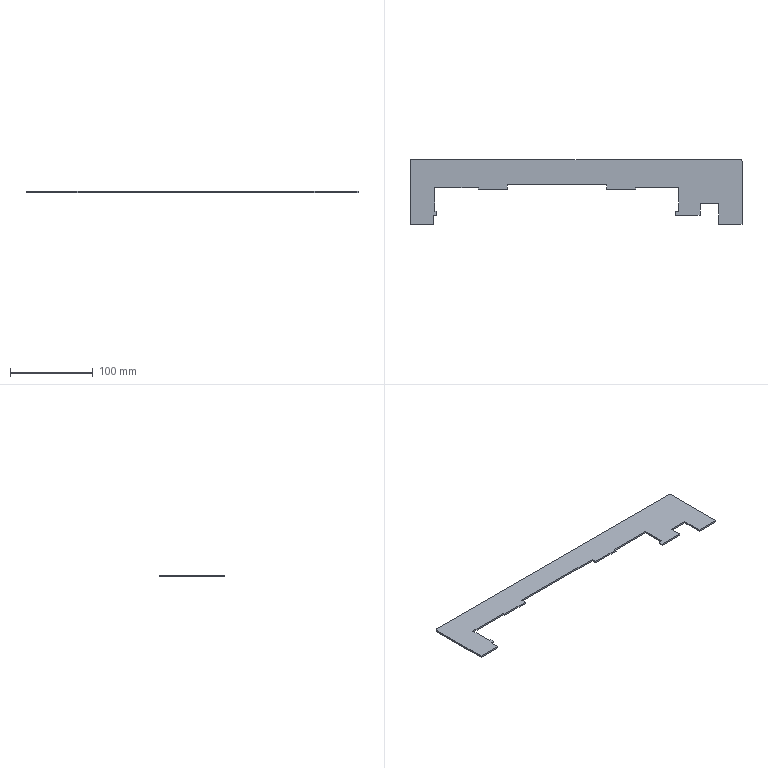Part | STEP file | xzz-001-1 | 1 solid | 30 faces | box 400 x 78 x 2 mm | volume 34179 mm3 | plane 28 | cylinder 2 | commonest cylinder face diameters 4 x2
STEP:
#1=CARTESIAN_POINT('',(221.,30.,0.));
#2=VERTEX_POINT('',#1);
#3=CARTESIAN_POINT('',(223.,28.,0.));
#4=VERTEX_POINT('',#3);
#5=CARTESIAN_POINT('',(221.,28.,0.));
#6=DIRECTION('',(0.,0.,-1.));
#7=DIRECTION('',(1.,0.,0.));
#8=AXIS2_PLACEMENT_3D('',#5,#6,#7);
#9=CIRCLE('',#8,2.);
#10=EDGE_CURVE('',#2,#4,#9,.T.);
#11=ORIENTED_EDGE('',*,*,#10,.F.);
#12=CARTESIAN_POINT('',(-175.,30.,0.));
#13=VERTEX_POINT('',#12);
#14=CARTESIAN_POINT('',(0.,30.,0.));
#15=DIRECTION('',(1.,0.,0.));
#16=VECTOR('',#15,1000.);
#17=LINE('',#14,#16);
#18=EDGE_CURVE('',#13,#2,#17,.T.);
#19=ORIENTED_EDGE('',*,*,#18,.F.);
#20=CARTESIAN_POINT('',(-177.,28.,0.));
#21=VERTEX_POINT('',#20);
#22=CARTESIAN_POINT('',(-175.,28.,0.));
#23=DIRECTION('',(0.,0.,-1.));
#24=DIRECTION('',(1.,0.,0.));
#25=AXIS2_PLACEMENT_3D('',#22,#23,#24);
#26=CIRCLE('',#25,2.);
#27=EDGE_CURVE('',#21,#13,#26,.T.);
#28=ORIENTED_EDGE('',*,*,#27,.F.);
#29=CARTESIAN_POINT('',(-177.,-48.,0.));
#30=VERTEX_POINT('',#29);
#31=CARTESIAN_POINT('',(-177.,0.,0.));
#32=DIRECTION('',(0.,1.,0.));
#33=VECTOR('',#32,1000.);
#34=LINE('',#31,#33);
#35=EDGE_CURVE('',#30,#21,#34,.T.);
#36=ORIENTED_EDGE('',*,*,#35,.F.);
#37=CARTESIAN_POINT('',(-149.,-48.,0.));
#38=VERTEX_POINT('',#37);
#39=CARTESIAN_POINT('',(0.,-48.,0.));
#40=DIRECTION('',(-1.,0.,0.));
#41=VECTOR('',#40,1000.);
#42=LINE('',#39,#41);
#43=EDGE_CURVE('',#38,#30,#42,.T.);
#44=ORIENTED_EDGE('',*,*,#43,.F.);
#45=CARTESIAN_POINT('',(-149.,-37.,0.));
#46=VERTEX_POINT('',#45);
#47=CARTESIAN_POINT('',(-149.,0.,0.));
#48=DIRECTION('',(0.,-1.,0.));
#49=VECTOR('',#48,1000.);
#50=LINE('',#47,#49);
#51=EDGE_CURVE('',#46,#38,#50,.T.);
#52=ORIENTED_EDGE('',*,*,#51,.F.);
#53=CARTESIAN_POINT('',(-145.,-37.,0.));
#54=VERTEX_POINT('',#53);
#55=CARTESIAN_POINT('',(0.,-37.,0.));
#56=DIRECTION('',(-1.,0.,0.));
#57=VECTOR('',#56,1000.);
#58=LINE('',#55,#57);
#59=EDGE_CURVE('',#54,#46,#58,.T.);
#60=ORIENTED_EDGE('',*,*,#59,.F.);
#61=CARTESIAN_POINT('',(-145.,-32.,0.));
#62=VERTEX_POINT('',#61);
#63=CARTESIAN_POINT('',(-145.,0.,0.));
#64=DIRECTION('',(0.,-1.,0.));
#65=VECTOR('',#64,1000.);
#66=LINE('',#63,#65);
#67=EDGE_CURVE('',#62,#54,#66,.T.);
#68=ORIENTED_EDGE('',*,*,#67,.F.);
#69=CARTESIAN_POINT('',(-147.,-32.,0.));
#70=VERTEX_POINT('',#69);
#71=CARTESIAN_POINT('',(0.,-32.,0.));
#72=DIRECTION('',(1.,0.,0.));
#73=VECTOR('',#72,1000.);
#74=LINE('',#71,#73);
#75=EDGE_CURVE('',#70,#62,#74,.T.);
#76=ORIENTED_EDGE('',*,*,#75,.F.);
#77=CARTESIAN_POINT('',(-147.,-4.,0.));
#78=VERTEX_POINT('',#77);
#79=CARTESIAN_POINT('',(-147.,0.,0.));
#80=DIRECTION('',(0.,-1.,0.));
#81=VECTOR('',#80,1000.);
#82=LINE('',#79,#81);
#83=EDGE_CURVE('',#78,#70,#82,.T.);
#84=ORIENTED_EDGE('',*,*,#83,.F.);
#85=CARTESIAN_POINT('',(-95.,-4.,0.));
#86=VERTEX_POINT('',#85);
#87=CARTESIAN_POINT('',(0.,-4.,0.));
#88=DIRECTION('',(-1.,0.,0.));
#89=VECTOR('',#88,1000.);
#90=LINE('',#87,#89);
#91=EDGE_CURVE('',#86,#78,#90,.T.);
#92=ORIENTED_EDGE('',*,*,#91,.F.);
#93=CARTESIAN_POINT('',(-95.,-6.,0.));
#94=VERTEX_POINT('',#93);
#95=CARTESIAN_POINT('',(-95.,0.,0.));
#96=DIRECTION('',(0.,1.,0.));
#97=VECTOR('',#96,1000.);
#98=LINE('',#95,#97);
#99=EDGE_CURVE('',#94,#86,#98,.T.);
#100=ORIENTED_EDGE('',*,*,#99,.F.);
#101=CARTESIAN_POINT('',(-60.,-6.,0.));
#102=VERTEX_POINT('',#101);
#103=CARTESIAN_POINT('',(0.,-6.,0.));
#104=DIRECTION('',(-1.,0.,0.));
#105=VECTOR('',#104,1000.);
#106=LINE('',#103,#105);
#107=EDGE_CURVE('',#102,#94,#106,.T.);
#108=ORIENTED_EDGE('',*,*,#107,.F.);
#109=CARTESIAN_POINT('',(-60.,0.000000001,0.));
#110=VERTEX_POINT('',#109);
#111=CARTESIAN_POINT('',(-60.,0.,0.));
#112=DIRECTION('',(0.,-1.,0.));
#113=VECTOR('',#112,1000.);
#114=LINE('',#111,#113);
#115=EDGE_CURVE('',#110,#102,#114,.T.);
#116=ORIENTED_EDGE('',*,*,#115,.F.);
#117=CARTESIAN_POINT('',(60.,0.000000001,0.));
#118=VERTEX_POINT('',#117);
#119=CARTESIAN_POINT('',(0.,0.000000001,0.));
#120=DIRECTION('',(-1.,0.,0.));
#121=VECTOR('',#120,1000.);
#122=LINE('',#119,#121);
#123=EDGE_CURVE('',#118,#110,#122,.T.);
#124=ORIENTED_EDGE('',*,*,#123,.F.);
#125=CARTESIAN_POINT('',(60.,-6.,0.));
#126=VERTEX_POINT('',#125);
#127=CARTESIAN_POINT('',(60.,0.,0.));
#128=DIRECTION('',(0.,1.,0.));
#129=VECTOR('',#128,1000.);
#130=LINE('',#127,#129);
#131=EDGE_CURVE('',#126,#118,#130,.T.);
#132=ORIENTED_EDGE('',*,*,#131,.F.);
#133=CARTESIAN_POINT('',(95.,-6.,0.));
#134=VERTEX_POINT('',#133);
#135=CARTESIAN_POINT('',(0.,-6.,0.));
#136=DIRECTION('',(-1.,0.,0.));
#137=VECTOR('',#136,1000.);
#138=LINE('',#135,#137);
#139=EDGE_CURVE('',#134,#126,#138,.T.);
#140=ORIENTED_EDGE('',*,*,#139,.F.);
#141=CARTESIAN_POINT('',(95.,-4.,0.));
#142=VERTEX_POINT('',#141);
#143=CARTESIAN_POINT('',(95.,0.,0.));
#144=DIRECTION('',(0.,-1.,0.));
#145=VECTOR('',#144,1000.);
#146=LINE('',#143,#145);
#147=EDGE_CURVE('',#142,#134,#146,.T.);
#148=ORIENTED_EDGE('',*,*,#147,.F.);
#149=CARTESIAN_POINT('',(147.,-4.,0.));
#150=VERTEX_POINT('',#149);
#151=CARTESIAN_POINT('',(0.,-4.,0.));
#152=DIRECTION('',(-1.,0.,0.));
#153=VECTOR('',#152,1000.);
#154=LINE('',#151,#153);
#155=EDGE_CURVE('',#150,#142,#154,.T.);
#156=ORIENTED_EDGE('',*,*,#155,.F.);
#157=CARTESIAN_POINT('',(147.,-32.,0.));
#158=VERTEX_POINT('',#157);
#159=CARTESIAN_POINT('',(147.,0.,0.));
#160=DIRECTION('',(0.,1.,0.));
#161=VECTOR('',#160,1000.);
#162=LINE('',#159,#161);
#163=EDGE_CURVE('',#158,#150,#162,.T.);
#164=ORIENTED_EDGE('',*,*,#163,.F.);
#165=CARTESIAN_POINT('',(142.454,-32.,0.));
#166=VERTEX_POINT('',#165);
#167=CARTESIAN_POINT('',(0.,-32.,0.));
#168=DIRECTION('',(1.,0.,0.));
#169=VECTOR('',#168,1000.);
#170=LINE('',#167,#169);
#171=EDGE_CURVE('',#166,#158,#170,.T.);
#172=ORIENTED_EDGE('',*,*,#171,.F.);
#173=CARTESIAN_POINT('',(142.454,-37.,0.));
#174=VERTEX_POINT('',#173);
#175=CARTESIAN_POINT('',(142.454,0.,0.));
#176=DIRECTION('',(0.,1.,0.));
#177=VECTOR('',#176,1000.);
#178=LINE('',#175,#177);
#179=EDGE_CURVE('',#174,#166,#178,.T.);
#180=ORIENTED_EDGE('',*,*,#179,.F.);
#181=CARTESIAN_POINT('',(172.454,-37.,0.));
#182=VERTEX_POINT('',#181);
#183=CARTESIAN_POINT('',(0.,-37.,0.));
#184=DIRECTION('',(-1.,0.,0.));
#185=VECTOR('',#184,1000.);
#186=LINE('',#183,#185);
#187=EDGE_CURVE('',#182,#174,#186,.T.);
#188=ORIENTED_EDGE('',*,*,#187,.F.);
#189=CARTESIAN_POINT('',(172.454,-23.,0.));
#190=VERTEX_POINT('',#189);
#191=CARTESIAN_POINT('',(172.454,0.,0.));
#192=DIRECTION('',(0.,-1.,0.));
#193=VECTOR('',#192,1000.);
#194=LINE('',#191,#193);
#195=EDGE_CURVE('',#190,#182,#194,.T.);
#196=ORIENTED_EDGE('',*,*,#195,.F.);
#197=CARTESIAN_POINT('',(195.,-23.,0.));
#198=VERTEX_POINT('',#197);
#199=CARTESIAN_POINT('',(0.,-23.,0.));
#200=DIRECTION('',(-1.,0.,0.));
#201=VECTOR('',#200,1000.);
#202=LINE('',#199,#201);
#203=EDGE_CURVE('',#198,#190,#202,.T.);
#204=ORIENTED_EDGE('',*,*,#203,.F.);
#205=CARTESIAN_POINT('',(195.,-48.,0.));
#206=VERTEX_POINT('',#205);
#207=CARTESIAN_POINT('',(195.,0.,0.));
#208=DIRECTION('',(0.,1.,0.));
#209=VECTOR('',#208,1000.);
#210=LINE('',#207,#209);
#211=EDGE_CURVE('',#206,#198,#210,.T.);
#212=ORIENTED_EDGE('',*,*,#211,.F.);
#213=CARTESIAN_POINT('',(223.,-48.,0.));
#214=VERTEX_POINT('',#213);
#215=CARTESIAN_POINT('',(0.,-48.,0.));
#216=DIRECTION('',(-1.,0.,0.));
#217=VECTOR('',#216,1000.);
#218=LINE('',#215,#217);
#219=EDGE_CURVE('',#214,#206,#218,.T.);
#220=ORIENTED_EDGE('',*,*,#219,.F.);
#221=CARTESIAN_POINT('',(223.,0.,0.));
#222=DIRECTION('',(0.,-1.,0.));
#223=VECTOR('',#222,1000.);
#224=LINE('',#221,#223);
#225=EDGE_CURVE('',#4,#214,#224,.T.);
#226=ORIENTED_EDGE('',*,*,#225,.F.);
#227=EDGE_LOOP('',(#11,#19,#28,#36,#44,#52,#60,#68,#76,#84,#92,#100,#108,#116,#124,#132,#140,#148,#156,#164,#172,#180,#188,#196,#204,#212,#220,#226));
#228=FACE_OUTER_BOUND('',#227,.T.);
#229=CARTESIAN_POINT('',(0.,0.,0.));
#230=DIRECTION('',(0.,0.,-1.));
#231=DIRECTION('',(-1.,0.,0.));
#232=AXIS2_PLACEMENT_3D('',#229,#230,#231);
#233=PLANE('',#232);
#234=ADVANCED_FACE('',(#228),#233,.F.);
#235=ORIENTED_EDGE('',*,*,#225,.T.);
#236=CARTESIAN_POINT('',(223.,-48.,-2.));
#237=VERTEX_POINT('',#236);
#238=CARTESIAN_POINT('',(223.,-48.,-2.));
#239=DIRECTION('',(0.,0.,-1.));
#240=VECTOR('',#239,1000.);
#241=LINE('',#238,#240);
#242=EDGE_CURVE('',#214,#237,#241,.T.);
#243=ORIENTED_EDGE('',*,*,#242,.T.);
#244=CARTESIAN_POINT('',(223.,28.,-2.));
#245=VERTEX_POINT('',#244);
#246=CARTESIAN_POINT('',(223.,30.,-2.));
#247=DIRECTION('',(0.,1.,0.));
#248=VECTOR('',#247,1000.);
#249=LINE('',#246,#248);
#250=EDGE_CURVE('',#237,#245,#249,.T.);
#251=ORIENTED_EDGE('',*,*,#250,.T.);
#252=CARTESIAN_POINT('',(223.,28.,-2.));
#253=DIRECTION('',(0.,0.,1.));
#254=VECTOR('',#253,1000.);
#255=LINE('',#252,#254);
#256=EDGE_CURVE('',#245,#4,#255,.T.);
#257=ORIENTED_EDGE('',*,*,#256,.T.);
#258=EDGE_LOOP('',(#235,#243,#251,#257));
#259=FACE_OUTER_BOUND('',#258,.T.);
#260=CARTESIAN_POINT('',(223.,30.,-2.));
#261=DIRECTION('',(1.,0.,0.));
#262=DIRECTION('',(0.,0.,-1.));
#263=AXIS2_PLACEMENT_3D('',#260,#261,#262);
#264=PLANE('',#263);
#265=ADVANCED_FACE('',(#259),#264,.T.);
#266=ORIENTED_EDGE('',*,*,#10,.T.);
#267=ORIENTED_EDGE('',*,*,#256,.F.);
#268=CARTESIAN_POINT('',(221.,30.,-2.));
#269=VERTEX_POINT('',#268);
#270=CARTESIAN_POINT('',(221.,28.,-2.));
#271=DIRECTION('',(0.,0.,1.));
#272=DIRECTION('',(1.,0.,0.));
#273=AXIS2_PLACEMENT_3D('',#270,#271,#272);
#274=CIRCLE('',#273,2.);
#275=EDGE_CURVE('',#245,#269,#274,.T.);
#276=ORIENTED_EDGE('',*,*,#275,.T.);
#277=CARTESIAN_POINT('',(221.,30.,-2.));
#278=DIRECTION('',(0.,0.,1.));
#279=VECTOR('',#278,1000.);
#280=LINE('',#277,#279);
#281=EDGE_CURVE('',#269,#2,#280,.T.);
#282=ORIENTED_EDGE('',*,*,#281,.T.);
#283=EDGE_LOOP('',(#266,#267,#276,#282));
#284=FACE_OUTER_BOUND('',#283,.T.);
#285=CARTESIAN_POINT('',(221.,28.,-2.));
#286=DIRECTION('',(0.,0.,1.));
#287=DIRECTION('',(1.,0.,0.));
#288=AXIS2_PLACEMENT_3D('',#285,#286,#287);
#289=CYLINDRICAL_SURFACE('',#288,2.);
#290=ADVANCED_FACE('',(#284),#289,.T.);
#291=CARTESIAN_POINT('',(-175.,30.,-2.));
#292=VERTEX_POINT('',#291);
#293=CARTESIAN_POINT('',(-177.,30.,-2.));
#294=DIRECTION('',(-1.,0.,0.));
#295=VECTOR('',#294,1000.);
#296=LINE('',#293,#295);
#297=EDGE_CURVE('',#269,#292,#296,.T.);
#298=ORIENTED_EDGE('',*,*,#297,.T.);
#299=CARTESIAN_POINT('',(-175.,30.,-2.));
#300=DIRECTION('',(0.,0.,1.));
#301=VECTOR('',#300,1000.);
#302=LINE('',#299,#301);
#303=EDGE_CURVE('',#292,#13,#302,.T.);
#304=ORIENTED_EDGE('',*,*,#303,.T.);
#305=ORIENTED_EDGE('',*,*,#18,.T.);
#306=ORIENTED_EDGE('',*,*,#281,.F.);
#307=EDGE_LOOP('',(#298,#304,#305,#306));
#308=FACE_OUTER_BOUND('',#307,.T.);
#309=CARTESIAN_POINT('',(-177.,30.,-2.));
#310=DIRECTION('',(0.,1.,0.));
#311=DIRECTION('',(0.,0.,1.));
#312=AXIS2_PLACEMENT_3D('',#309,#310,#311);
#313=PLANE('',#312);
#314=ADVANCED_FACE('',(#308),#313,.T.);
#315=ORIENTED_EDGE('',*,*,#27,.T.);
#316=ORIENTED_EDGE('',*,*,#303,.F.);
#317=CARTESIAN_POINT('',(-177.,28.,-2.));
#318=VERTEX_POINT('',#317);
#319=CARTESIAN_POINT('',(-175.,28.,-2.));
#320=DIRECTION('',(0.,0.,1.));
#321=DIRECTION('',(1.,0.,0.));
#322=AXIS2_PLACEMENT_3D('',#319,#320,#321);
#323=CIRCLE('',#322,2.);
#324=EDGE_CURVE('',#292,#318,#323,.T.);
#325=ORIENTED_EDGE('',*,*,#324,.T.);
#326=CARTESIAN_POINT('',(-177.,28.,-2.));
#327=DIRECTION('',(0.,0.,1.));
#328=VECTOR('',#327,1000.);
#329=LINE('',#326,#328);
#330=EDGE_CURVE('',#318,#21,#329,.T.);
#331=ORIENTED_EDGE('',*,*,#330,.T.);
#332=EDGE_LOOP('',(#315,#316,#325,#331));
#333=FACE_OUTER_BOUND('',#332,.T.);
#334=CARTESIAN_POINT('',(-175.,28.,-2.));
#335=DIRECTION('',(0.,0.,1.));
#336=DIRECTION('',(1.,0.,0.));
#337=AXIS2_PLACEMENT_3D('',#334,#335,#336);
#338=CYLINDRICAL_SURFACE('',#337,2.);
#339=ADVANCED_FACE('',(#333),#338,.T.);
#340=CARTESIAN_POINT('',(-177.,-48.,-2.));
#341=VERTEX_POINT('',#340);
#342=CARTESIAN_POINT('',(-177.,30.,-2.));
#343=DIRECTION('',(0.,-1.,0.));
#344=VECTOR('',#343,1000.);
#345=LINE('',#342,#344);
#346=EDGE_CURVE('',#318,#341,#345,.T.);
#347=ORIENTED_EDGE('',*,*,#346,.T.);
#348=CARTESIAN_POINT('',(-177.,-48.,-2.));
#349=DIRECTION('',(0.,0.,1.));
#350=VECTOR('',#349,1000.);
#351=LINE('',#348,#350);
#352=EDGE_CURVE('',#341,#30,#351,.T.);
#353=ORIENTED_EDGE('',*,*,#352,.T.);
#354=ORIENTED_EDGE('',*,*,#35,.T.);
#355=ORIENTED_EDGE('',*,*,#330,.F.);
#356=EDGE_LOOP('',(#347,#353,#354,#355));
#357=FACE_OUTER_BOUND('',#356,.T.);
#358=CARTESIAN_POINT('',(-177.,30.,-2.));
#359=DIRECTION('',(-1.,0.,0.));
#360=DIRECTION('',(0.,0.,1.));
#361=AXIS2_PLACEMENT_3D('',#358,#359,#360);
#362=PLANE('',#361);
#363=ADVANCED_FACE('',(#357),#362,.T.);
#364=CARTESIAN_POINT('',(-149.,-48.,-2.));
#365=VERTEX_POINT('',#364);
#366=CARTESIAN_POINT('',(-177.,-48.,-2.));
#367=DIRECTION('',(1.,0.,0.));
#368=VECTOR('',#367,1000.);
#369=LINE('',#366,#368);
#370=EDGE_CURVE('',#341,#365,#369,.T.);
#371=ORIENTED_EDGE('',*,*,#370,.T.);
#372=CARTESIAN_POINT('',(-149.,-48.,-2.));
#373=DIRECTION('',(0.,0.,1.));
#374=VECTOR('',#373,1000.);
#375=LINE('',#372,#374);
#376=EDGE_CURVE('',#365,#38,#375,.T.);
#377=ORIENTED_EDGE('',*,*,#376,.T.);
#378=ORIENTED_EDGE('',*,*,#43,.T.);
#379=ORIENTED_EDGE('',*,*,#352,.F.);
#380=EDGE_LOOP('',(#371,#377,#378,#379));
#381=FACE_OUTER_BOUND('',#380,.T.);
#382=CARTESIAN_POINT('',(-177.,-48.,-2.));
#383=DIRECTION('',(0.,-1.,0.));
#384=DIRECTION('',(1.,0.,0.));
#385=AXIS2_PLACEMENT_3D('',#382,#383,#384);
#386=PLANE('',#385);
#387=ADVANCED_FACE('',(#381),#386,.T.);
#388=CARTESIAN_POINT('',(-149.,-37.,-2.));
#389=VERTEX_POINT('',#388);
#390=CARTESIAN_POINT('',(-149.,-48.,-2.));
#391=DIRECTION('',(0.,1.,0.));
#392=VECTOR('',#391,1000.);
#393=LINE('',#390,#392);
#394=EDGE_CURVE('',#365,#389,#393,.T.);
#395=ORIENTED_EDGE('',*,*,#394,.T.);
#396=CARTESIAN_POINT('',(-149.,-37.,-2.));
#397=DIRECTION('',(0.,0.,1.));
#398=VECTOR('',#397,1000.);
#399=LINE('',#396,#398);
#400=EDGE_CURVE('',#389,#46,#399,.T.);
#401=ORIENTED_EDGE('',*,*,#400,.T.);
#402=ORIENTED_EDGE('',*,*,#51,.T.);
#403=ORIENTED_EDGE('',*,*,#376,.F.);
#404=EDGE_LOOP('',(#395,#401,#402,#403));
#405=FACE_OUTER_BOUND('',#404,.T.);
#406=CARTESIAN_POINT('',(-149.,-48.,-2.));
#407=DIRECTION('',(1.,0.,0.));
#408=DIRECTION('',(0.,0.,-1.));
#409=AXIS2_PLACEMENT_3D('',#406,#407,#408);
#410=PLANE('',#409);
#411=ADVANCED_FACE('',(#405),#410,.T.);
#412=CARTESIAN_POINT('',(-145.,-37.,-2.));
#413=VERTEX_POINT('',#412);
#414=CARTESIAN_POINT('',(-145.,-37.,-2.));
#415=DIRECTION('',(1.,0.,0.));
#416=VECTOR('',#415,1000.);
#417=LINE('',#414,#416);
#418=EDGE_CURVE('',#389,#413,#417,.T.);
#419=ORIENTED_EDGE('',*,*,#418,.T.);
#420=CARTESIAN_POINT('',(-145.,-37.,-2.));
#421=DIRECTION('',(0.,0.,1.));
#422=VECTOR('',#421,1000.);
#423=LINE('',#420,#422);
#424=EDGE_CURVE('',#413,#54,#423,.T.);
#425=ORIENTED_EDGE('',*,*,#424,.T.);
#426=ORIENTED_EDGE('',*,*,#59,.T.);
#427=ORIENTED_EDGE('',*,*,#400,.F.);
#428=EDGE_LOOP('',(#419,#425,#426,#427));
#429=FACE_OUTER_BOUND('',#428,.T.);
#430=CARTESIAN_POINT('',(-145.,-37.,-2.));
#431=DIRECTION('',(0.,-1.,0.));
#432=DIRECTION('',(0.,0.,-1.));
#433=AXIS2_PLACEMENT_3D('',#430,#431,#432);
#434=PLANE('',#433);
#435=ADVANCED_FACE('',(#429),#434,.T.);
#436=CARTESIAN_POINT('',(-145.,-32.,-2.));
#437=VERTEX_POINT('',#436);
#438=CARTESIAN_POINT('',(-145.,-32.,-2.));
#439=DIRECTION('',(0.,1.,0.));
#440=VECTOR('',#439,1000.);
#441=LINE('',#438,#440);
#442=EDGE_CURVE('',#413,#437,#441,.T.);
#443=ORIENTED_EDGE('',*,*,#442,.T.);
#444=CARTESIAN_POINT('',(-145.,-32.,-2.));
#445=DIRECTION('',(0.,0.,1.));
#446=VECTOR('',#445,1000.);
#447=LINE('',#444,#446);
#448=EDGE_CURVE('',#437,#62,#447,.T.);
#449=ORIENTED_EDGE('',*,*,#448,.T.);
#450=ORIENTED_EDGE('',*,*,#67,.T.);
#451=ORIENTED_EDGE('',*,*,#424,.F.);
#452=EDGE_LOOP('',(#443,#449,#450,#451));
#453=FACE_OUTER_BOUND('',#452,.T.);
#454=CARTESIAN_POINT('',(-145.,-32.,-2.));
#455=DIRECTION('',(1.,0.,0.));
#456=DIRECTION('',(0.,0.,-1.));
#457=AXIS2_PLACEMENT_3D('',#454,#455,#456);
#458=PLANE('',#457);
#459=ADVANCED_FACE('',(#453),#458,.T.);
#460=CARTESIAN_POINT('',(-147.,-32.,-2.));
#461=VERTEX_POINT('',#460);
#462=CARTESIAN_POINT('',(-147.,-32.,-2.));
#463=DIRECTION('',(-1.,0.,0.));
#464=VECTOR('',#463,1000.);
#465=LINE('',#462,#464);
#466=EDGE_CURVE('',#437,#461,#465,.T.);
#467=ORIENTED_EDGE('',*,*,#466,.T.);
#468=CARTESIAN_POINT('',(-147.,-32.,-2.));
#469=DIRECTION('',(0.,0.,1.));
#470=VECTOR('',#469,1000.);
#471=LINE('',#468,#470);
#472=EDGE_CURVE('',#461,#70,#471,.T.);
#473=ORIENTED_EDGE('',*,*,#472,.T.);
#474=ORIENTED_EDGE('',*,*,#75,.T.);
#475=ORIENTED_EDGE('',*,*,#448,.F.);
#476=EDGE_LOOP('',(#467,#473,#474,#475));
#477=FACE_OUTER_BOUND('',#476,.T.);
#478=CARTESIAN_POINT('',(-147.,-32.,-2.));
#479=DIRECTION('',(0.,1.,0.));
#480=DIRECTION('',(0.,0.,1.));
#481=AXIS2_PLACEMENT_3D('',#478,#479,#480);
#482=PLANE('',#481);
#483=ADVANCED_FACE('',(#477),#482,.T.);
#484=CARTESIAN_POINT('',(-147.,-4.,-2.));
#485=VERTEX_POINT('',#484);
#486=CARTESIAN_POINT('',(-147.,-32.,-2.));
#487=DIRECTION('',(0.,1.,0.));
#488=VECTOR('',#487,1000.);
#489=LINE('',#486,#488);
#490=EDGE_CURVE('',#461,#485,#489,.T.);
#491=ORIENTED_EDGE('',*,*,#490,.T.);
#492=CARTESIAN_POINT('',(-147.,-4.,-2.));
#493=DIRECTION('',(0.,0.,1.));
#494=VECTOR('',#493,1000.);
#495=LINE('',#492,#494);
#496=EDGE_CURVE('',#485,#78,#495,.T.);
#497=ORIENTED_EDGE('',*,*,#496,.T.);
#498=ORIENTED_EDGE('',*,*,#83,.T.);
#499=ORIENTED_EDGE('',*,*,#472,.F.);
#500=EDGE_LOOP('',(#491,#497,#498,#499));
#501=FACE_OUTER_BOUND('',#500,.T.);
#502=CARTESIAN_POINT('',(-147.,-32.,-2.));
#503=DIRECTION('',(1.,0.,0.));
#504=DIRECTION('',(0.,0.,-1.));
#505=AXIS2_PLACEMENT_3D('',#502,#503,#504);
#506=PLANE('',#505);
#507=ADVANCED_FACE('',(#501),#506,.T.);
#508=CARTESIAN_POINT('',(-95.,-4.,-2.));
#509=VERTEX_POINT('',#508);
#510=CARTESIAN_POINT('',(-147.,-4.,-2.));
#511=DIRECTION('',(1.,0.,0.));
#512=VECTOR('',#511,1000.);
#513=LINE('',#510,#512);
#514=EDGE_CURVE('',#485,#509,#513,.T.);
#515=ORIENTED_EDGE('',*,*,#514,.T.);
#516=CARTESIAN_POINT('',(-95.,-4.,-2.));
#517=DIRECTION('',(0.,0.,1.));
#518=VECTOR('',#517,1000.);
#519=LINE('',#516,#518);
#520=EDGE_CURVE('',#509,#86,#519,.T.);
#521=ORIENTED_EDGE('',*,*,#520,.T.);
#522=ORIENTED_EDGE('',*,*,#91,.T.);
#523=ORIENTED_EDGE('',*,*,#496,.F.);
#524=EDGE_LOOP('',(#515,#521,#522,#523));
#525=FACE_OUTER_BOUND('',#524,.T.);
#526=CARTESIAN_POINT('',(-147.,-4.,-2.));
#527=DIRECTION('',(0.,-1.,0.));
#528=DIRECTION('',(0.,0.,-1.));
#529=AXIS2_PLACEMENT_3D('',#526,#527,#528);
#530=PLANE('',#529);
#531=ADVANCED_FACE('',(#525),#530,.T.);
#532=CARTESIAN_POINT('',(-95.,-6.,-2.));
#533=VERTEX_POINT('',#532);
#534=CARTESIAN_POINT('',(-95.,-4.,-2.));
#535=DIRECTION('',(0.,-1.,0.));
#536=VECTOR('',#535,1000.);
#537=LINE('',#534,#536);
#538=EDGE_CURVE('',#509,#533,#537,.T.);
#539=ORIENTED_EDGE('',*,*,#538,.T.);
#540=CARTESIAN_POINT('',(-95.,-6.,-2.));
#541=DIRECTION('',(0.,0.,1.));
#542=VECTOR('',#541,1000.);
#543=LINE('',#540,#542);
#544=EDGE_CURVE('',#533,#94,#543,.T.);
#545=ORIENTED_EDGE('',*,*,#544,.T.);
#546=ORIENTED_EDGE('',*,*,#99,.T.);
#547=ORIENTED_EDGE('',*,*,#520,.F.);
#548=EDGE_LOOP('',(#539,#545,#546,#547));
#549=FACE_OUTER_BOUND('',#548,.T.);
#550=CARTESIAN_POINT('',(-95.,-4.,-2.));
#551=DIRECTION('',(-1.,0.,0.));
#552=DIRECTION('',(0.,0.,1.));
#553=AXIS2_PLACEMENT_3D('',#550,#551,#552);
#554=PLANE('',#553);
#555=ADVANCED_FACE('',(#549),#554,.T.);
#556=CARTESIAN_POINT('',(-60.,-6.,-2.));
#557=VERTEX_POINT('',#556);
#558=CARTESIAN_POINT('',(-95.,-6.,-2.));
#559=DIRECTION('',(1.,0.,0.));
#560=VECTOR('',#559,1000.);
#561=LINE('',#558,#560);
#562=EDGE_CURVE('',#533,#557,#561,.T.);
#563=ORIENTED_EDGE('',*,*,#562,.T.);
#564=CARTESIAN_POINT('',(-60.,-6.,-2.));
#565=DIRECTION('',(0.,0.,1.));
#566=VECTOR('',#565,1000.);
#567=LINE('',#564,#566);
#568=EDGE_CURVE('',#557,#102,#567,.T.);
#569=ORIENTED_EDGE('',*,*,#568,.T.);
#570=ORIENTED_EDGE('',*,*,#107,.T.);
#571=ORIENTED_EDGE('',*,*,#544,.F.);
#572=EDGE_LOOP('',(#563,#569,#570,#571));
#573=FACE_OUTER_BOUND('',#572,.T.);
#574=CARTESIAN_POINT('',(-95.,-6.,-2.));
#575=DIRECTION('',(0.,-1.,0.));
#576=DIRECTION('',(0.,0.,-1.));
#577=AXIS2_PLACEMENT_3D('',#574,#575,#576);
#578=PLANE('',#577);
#579=ADVANCED_FACE('',(#573),#578,.T.);
#580=CARTESIAN_POINT('',(-60.,0.000000001,-2.));
#581=VERTEX_POINT('',#580);
#582=CARTESIAN_POINT('',(-60.,-6.,-2.));
#583=DIRECTION('',(0.,1.,0.));
#584=VECTOR('',#583,1000.);
#585=LINE('',#582,#584);
#586=EDGE_CURVE('',#557,#581,#585,.T.);
#587=ORIENTED_EDGE('',*,*,#586,.T.);
#588=CARTESIAN_POINT('',(-60.,0.000000001,-2.));
#589=DIRECTION('',(0.,0.,1.));
#590=VECTOR('',#589,1000.);
#591=LINE('',#588,#590);
#592=EDGE_CURVE('',#581,#110,#591,.T.);
#593=ORIENTED_EDGE('',*,*,#592,.T.);
#594=ORIENTED_EDGE('',*,*,#115,.T.);
#595=ORIENTED_EDGE('',*,*,#568,.F.);
#596=EDGE_LOOP('',(#587,#593,#594,#595));
#597=FACE_OUTER_BOUND('',#596,.T.);
#598=CARTESIAN_POINT('',(-60.,-6.,-2.));
#599=DIRECTION('',(1.,0.,0.));
#600=DIRECTION('',(0.,0.,-1.));
#601=AXIS2_PLACEMENT_3D('',#598,#599,#600);
#602=PLANE('',#601);
#603=ADVANCED_FACE('',(#597),#602,.T.);
#604=CARTESIAN_POINT('',(60.,0.000000001,-2.));
#605=VERTEX_POINT('',#604);
#606=CARTESIAN_POINT('',(-60.,0.000000001,-2.));
#607=DIRECTION('',(1.,0.,0.));
#608=VECTOR('',#607,1000.);
#609=LINE('',#606,#608);
#610=EDGE_CURVE('',#581,#605,#609,.T.);
#611=ORIENTED_EDGE('',*,*,#610,.T.);
#612=CARTESIAN_POINT('',(60.,0.000000001,-2.));
#613=DIRECTION('',(0.,0.,1.));
#614=VECTOR('',#613,1000.);
#615=LINE('',#612,#614);
#616=EDGE_CURVE('',#605,#118,#615,.T.);
#617=ORIENTED_EDGE('',*,*,#616,.T.);
#618=ORIENTED_EDGE('',*,*,#123,.T.);
#619=ORIENTED_EDGE('',*,*,#592,.F.);
#620=EDGE_LOOP('',(#611,#617,#618,#619));
#621=FACE_OUTER_BOUND('',#620,.T.);
#622=CARTESIAN_POINT('',(-60.,0.000000001,-2.));
#623=DIRECTION('',(0.,-1.,0.));
#624=DIRECTION('',(1.,0.,0.));
#625=AXIS2_PLACEMENT_3D('',#622,#623,#624);
#626=PLANE('',#625);
#627=ADVANCED_FACE('',(#621),#626,.T.);
#628=CARTESIAN_POINT('',(60.,-6.,-2.));
#629=VERTEX_POINT('',#628);
#630=CARTESIAN_POINT('',(60.,0.000000001,-2.));
#631=DIRECTION('',(0.,-1.,0.));
#632=VECTOR('',#631,1000.);
#633=LINE('',#630,#632);
#634=EDGE_CURVE('',#605,#629,#633,.T.);
#635=ORIENTED_EDGE('',*,*,#634,.T.);
#636=CARTESIAN_POINT('',(60.,-6.,-2.));
#637=DIRECTION('',(0.,0.,1.));
#638=VECTOR('',#637,1000.);
#639=LINE('',#636,#638);
#640=EDGE_CURVE('',#629,#126,#639,.T.);
#641=ORIENTED_EDGE('',*,*,#640,.T.);
#642=ORIENTED_EDGE('',*,*,#131,.T.);
#643=ORIENTED_EDGE('',*,*,#616,.F.);
#644=EDGE_LOOP('',(#635,#641,#642,#643));
#645=FACE_OUTER_BOUND('',#644,.T.);
#646=CARTESIAN_POINT('',(60.,0.000000001,-2.));
#647=DIRECTION('',(-1.,0.,0.));
#648=DIRECTION('',(0.,0.,1.));
#649=AXIS2_PLACEMENT_3D('',#646,#647,#648);
#650=PLANE('',#649);
#651=ADVANCED_FACE('',(#645),#650,.T.);
#652=CARTESIAN_POINT('',(95.,-6.,-2.));
#653=VERTEX_POINT('',#652);
#654=CARTESIAN_POINT('',(95.,-6.,-2.));
#655=DIRECTION('',(1.,0.,0.));
#656=VECTOR('',#655,1000.);
#657=LINE('',#654,#656);
#658=EDGE_CURVE('',#629,#653,#657,.T.);
#659=ORIENTED_EDGE('',*,*,#658,.T.);
#660=CARTESIAN_POINT('',(95.,-6.,-2.));
#661=DIRECTION('',(0.,0.,1.));
#662=VECTOR('',#661,1000.);
#663=LINE('',#660,#662);
#664=EDGE_CURVE('',#653,#134,#663,.T.);
#665=ORIENTED_EDGE('',*,*,#664,.T.);
#666=ORIENTED_EDGE('',*,*,#139,.T.);
#667=ORIENTED_EDGE('',*,*,#640,.F.);
#668=EDGE_LOOP('',(#659,#665,#666,#667));
#669=FACE_OUTER_BOUND('',#668,.T.);
#670=CARTESIAN_POINT('',(95.,-6.,-2.));
#671=DIRECTION('',(0.,-1.,0.));
#672=DIRECTION('',(1.,0.,0.));
#673=AXIS2_PLACEMENT_3D('',#670,#671,#672);
#674=PLANE('',#673);
#675=ADVANCED_FACE('',(#669),#674,.T.);
#676=CARTESIAN_POINT('',(95.,-4.,-2.));
#677=VERTEX_POINT('',#676);
#678=CARTESIAN_POINT('',(95.,-6.,-2.));
#679=DIRECTION('',(0.,1.,0.));
#680=VECTOR('',#679,1000.);
#681=LINE('',#678,#680);
#682=EDGE_CURVE('',#653,#677,#681,.T.);
#683=ORIENTED_EDGE('',*,*,#682,.T.);
#684=CARTESIAN_POINT('',(95.,-4.,-2.));
#685=DIRECTION('',(0.,0.,1.));
#686=VECTOR('',#685,1000.);
#687=LINE('',#684,#686);
#688=EDGE_CURVE('',#677,#142,#687,.T.);
#689=ORIENTED_EDGE('',*,*,#688,.T.);
#690=ORIENTED_EDGE('',*,*,#147,.T.);
#691=ORIENTED_EDGE('',*,*,#664,.F.);
#692=EDGE_LOOP('',(#683,#689,#690,#691));
#693=FACE_OUTER_BOUND('',#692,.T.);
#694=CARTESIAN_POINT('',(95.,-6.,-2.));
#695=DIRECTION('',(1.,0.,0.));
#696=DIRECTION('',(0.,0.,-1.));
#697=AXIS2_PLACEMENT_3D('',#694,#695,#696);
#698=PLANE('',#697);
#699=ADVANCED_FACE('',(#693),#698,.T.);
#700=CARTESIAN_POINT('',(147.,-4.,-2.));
#701=VERTEX_POINT('',#700);
#702=CARTESIAN_POINT('',(95.,-4.,-2.));
#703=DIRECTION('',(1.,0.,0.));
#704=VECTOR('',#703,1000.);
#705=LINE('',#702,#704);
#706=EDGE_CURVE('',#677,#701,#705,.T.);
#707=ORIENTED_EDGE('',*,*,#706,.T.);
#708=CARTESIAN_POINT('',(147.,-4.,-2.));
#709=DIRECTION('',(0.,0.,1.));
#710=VECTOR('',#709,1000.);
#711=LINE('',#708,#710);
#712=EDGE_CURVE('',#701,#150,#711,.T.);
#713=ORIENTED_EDGE('',*,*,#712,.T.);
#714=ORIENTED_EDGE('',*,*,#155,.T.);
#715=ORIENTED_EDGE('',*,*,#688,.F.);
#716=EDGE_LOOP('',(#707,#713,#714,#715));
#717=FACE_OUTER_BOUND('',#716,.T.);
#718=CARTESIAN_POINT('',(95.,-4.,-2.));
#719=DIRECTION('',(0.,-1.,0.));
#720=DIRECTION('',(0.,0.,-1.));
#721=AXIS2_PLACEMENT_3D('',#718,#719,#720);
#722=PLANE('',#721);
#723=ADVANCED_FACE('',(#717),#722,.T.);
#724=CARTESIAN_POINT('',(147.,-32.,-2.));
#725=VERTEX_POINT('',#724);
#726=CARTESIAN_POINT('',(147.,-4.,-2.));
#727=DIRECTION('',(0.,-1.,0.));
#728=VECTOR('',#727,1000.);
#729=LINE('',#726,#728);
#730=EDGE_CURVE('',#701,#725,#729,.T.);
#731=ORIENTED_EDGE('',*,*,#730,.T.);
#732=CARTESIAN_POINT('',(147.,-32.,-2.));
#733=DIRECTION('',(0.,0.,1.));
#734=VECTOR('',#733,1000.);
#735=LINE('',#732,#734);
#736=EDGE_CURVE('',#725,#158,#735,.T.);
#737=ORIENTED_EDGE('',*,*,#736,.T.);
#738=ORIENTED_EDGE('',*,*,#163,.T.);
#739=ORIENTED_EDGE('',*,*,#712,.F.);
#740=EDGE_LOOP('',(#731,#737,#738,#739));
#741=FACE_OUTER_BOUND('',#740,.T.);
#742=CARTESIAN_POINT('',(147.,-4.,-2.));
#743=DIRECTION('',(-1.,0.,0.));
#744=DIRECTION('',(0.,0.,1.));
#745=AXIS2_PLACEMENT_3D('',#742,#743,#744);
#746=PLANE('',#745);
#747=ADVANCED_FACE('',(#741),#746,.T.);
#748=CARTESIAN_POINT('',(142.454,-32.,-2.));
#749=VERTEX_POINT('',#748);
#750=CARTESIAN_POINT('',(147.,-32.,-2.));
#751=DIRECTION('',(-1.,0.,0.));
#752=VECTOR('',#751,1000.);
#753=LINE('',#750,#752);
#754=EDGE_CURVE('',#725,#749,#753,.T.);
#755=ORIENTED_EDGE('',*,*,#754,.T.);
#756=CARTESIAN_POINT('',(142.454,-32.,-2.));
#757=DIRECTION('',(0.,0.,1.));
#758=VECTOR('',#757,1000.);
#759=LINE('',#756,#758);
#760=EDGE_CURVE('',#749,#166,#759,.T.);
#761=ORIENTED_EDGE('',*,*,#760,.T.);
#762=ORIENTED_EDGE('',*,*,#171,.T.);
#763=ORIENTED_EDGE('',*,*,#736,.F.);
#764=EDGE_LOOP('',(#755,#761,#762,#763));
#765=FACE_OUTER_BOUND('',#764,.T.);
#766=CARTESIAN_POINT('',(147.,-32.,-2.));
#767=DIRECTION('',(0.,1.,0.));
#768=DIRECTION('',(0.,0.,1.));
#769=AXIS2_PLACEMENT_3D('',#766,#767,#768);
#770=PLANE('',#769);
#771=ADVANCED_FACE('',(#765),#770,.T.);
#772=CARTESIAN_POINT('',(142.454,-37.,-2.));
#773=VERTEX_POINT('',#772);
#774=CARTESIAN_POINT('',(142.454,-32.,-2.));
#775=DIRECTION('',(0.,-1.,0.));
#776=VECTOR('',#775,1000.);
#777=LINE('',#774,#776);
#778=EDGE_CURVE('',#749,#773,#777,.T.);
#779=ORIENTED_EDGE('',*,*,#778,.T.);
#780=CARTESIAN_POINT('',(142.454,-37.,-2.));
#781=DIRECTION('',(0.,0.,1.));
#782=VECTOR('',#781,1000.);
#783=LINE('',#780,#782);
#784=EDGE_CURVE('',#773,#174,#783,.T.);
#785=ORIENTED_EDGE('',*,*,#784,.T.);
#786=ORIENTED_EDGE('',*,*,#179,.T.);
#787=ORIENTED_EDGE('',*,*,#760,.F.);
#788=EDGE_LOOP('',(#779,#785,#786,#787));
#789=FACE_OUTER_BOUND('',#788,.T.);
#790=CARTESIAN_POINT('',(142.454,-32.,-2.));
#791=DIRECTION('',(-1.,0.,0.));
#792=DIRECTION('',(0.,0.,1.));
#793=AXIS2_PLACEMENT_3D('',#790,#791,#792);
#794=PLANE('',#793);
#795=ADVANCED_FACE('',(#789),#794,.T.);
#796=CARTESIAN_POINT('',(172.454,-37.,-2.));
#797=VERTEX_POINT('',#796);
#798=CARTESIAN_POINT('',(142.454,-37.,-2.));
#799=DIRECTION('',(1.,0.,0.));
#800=VECTOR('',#799,1000.);
#801=LINE('',#798,#800);
#802=EDGE_CURVE('',#773,#797,#801,.T.);
#803=ORIENTED_EDGE('',*,*,#802,.T.);
#804=CARTESIAN_POINT('',(172.454,-37.,-2.));
#805=DIRECTION('',(0.,0.,1.));
#806=VECTOR('',#805,1000.);
#807=LINE('',#804,#806);
#808=EDGE_CURVE('',#797,#182,#807,.T.);
#809=ORIENTED_EDGE('',*,*,#808,.T.);
#810=ORIENTED_EDGE('',*,*,#187,.T.);
#811=ORIENTED_EDGE('',*,*,#784,.F.);
#812=EDGE_LOOP('',(#803,#809,#810,#811));
#813=FACE_OUTER_BOUND('',#812,.T.);
#814=CARTESIAN_POINT('',(142.454,-37.,-2.));
#815=DIRECTION('',(0.,-1.,0.));
#816=DIRECTION('',(1.,0.,0.));
#817=AXIS2_PLACEMENT_3D('',#814,#815,#816);
#818=PLANE('',#817);
#819=ADVANCED_FACE('',(#813),#818,.T.);
#820=CARTESIAN_POINT('',(172.454,-23.,-2.));
#821=VERTEX_POINT('',#820);
#822=CARTESIAN_POINT('',(172.454,-37.,-2.));
#823=DIRECTION('',(0.,1.,0.));
#824=VECTOR('',#823,1000.);
#825=LINE('',#822,#824);
#826=EDGE_CURVE('',#797,#821,#825,.T.);
#827=ORIENTED_EDGE('',*,*,#826,.T.);
#828=CARTESIAN_POINT('',(172.454,-23.,-2.));
#829=DIRECTION('',(0.,0.,1.));
#830=VECTOR('',#829,1000.);
#831=LINE('',#828,#830);
#832=EDGE_CURVE('',#821,#190,#831,.T.);
#833=ORIENTED_EDGE('',*,*,#832,.T.);
#834=ORIENTED_EDGE('',*,*,#195,.T.);
#835=ORIENTED_EDGE('',*,*,#808,.F.);
#836=EDGE_LOOP('',(#827,#833,#834,#835));
#837=FACE_OUTER_BOUND('',#836,.T.);
#838=CARTESIAN_POINT('',(172.454,-37.,-2.));
#839=DIRECTION('',(1.,0.,0.));
#840=DIRECTION('',(0.,0.,-1.));
#841=AXIS2_PLACEMENT_3D('',#838,#839,#840);
#842=PLANE('',#841);
#843=ADVANCED_FACE('',(#837),#842,.T.);
#844=CARTESIAN_POINT('',(195.,-23.,-2.));
#845=VERTEX_POINT('',#844);
#846=CARTESIAN_POINT('',(172.454,-23.,-2.));
#847=DIRECTION('',(1.,0.,0.));
#848=VECTOR('',#847,1000.);
#849=LINE('',#846,#848);
#850=EDGE_CURVE('',#821,#845,#849,.T.);
#851=ORIENTED_EDGE('',*,*,#850,.T.);
#852=CARTESIAN_POINT('',(195.,-23.,-2.));
#853=DIRECTION('',(0.,0.,1.));
#854=VECTOR('',#853,1000.);
#855=LINE('',#852,#854);
#856=EDGE_CURVE('',#845,#198,#855,.T.);
#857=ORIENTED_EDGE('',*,*,#856,.T.);
#858=ORIENTED_EDGE('',*,*,#203,.T.);
#859=ORIENTED_EDGE('',*,*,#832,.F.);
#860=EDGE_LOOP('',(#851,#857,#858,#859));
#861=FACE_OUTER_BOUND('',#860,.T.);
#862=CARTESIAN_POINT('',(172.454,-23.,-2.));
#863=DIRECTION('',(0.,-1.,0.));
#864=DIRECTION('',(0.,0.,-1.));
#865=AXIS2_PLACEMENT_3D('',#862,#863,#864);
#866=PLANE('',#865);
#867=ADVANCED_FACE('',(#861),#866,.T.);
#868=CARTESIAN_POINT('',(195.,-48.,-2.));
#869=VERTEX_POINT('',#868);
#870=CARTESIAN_POINT('',(195.,-23.,-2.));
#871=DIRECTION('',(0.,-1.,0.));
#872=VECTOR('',#871,1000.);
#873=LINE('',#870,#872);
#874=EDGE_CURVE('',#845,#869,#873,.T.);
#875=ORIENTED_EDGE('',*,*,#874,.T.);
#876=CARTESIAN_POINT('',(195.,-48.,-2.));
#877=DIRECTION('',(0.,0.,1.));
#878=VECTOR('',#877,1000.);
#879=LINE('',#876,#878);
#880=EDGE_CURVE('',#869,#206,#879,.T.);
#881=ORIENTED_EDGE('',*,*,#880,.T.);
#882=ORIENTED_EDGE('',*,*,#211,.T.);
#883=ORIENTED_EDGE('',*,*,#856,.F.);
#884=EDGE_LOOP('',(#875,#881,#882,#883));
#885=FACE_OUTER_BOUND('',#884,.T.);
#886=CARTESIAN_POINT('',(195.,-23.,-2.));
#887=DIRECTION('',(-1.,0.,0.));
#888=DIRECTION('',(0.,0.,1.));
#889=AXIS2_PLACEMENT_3D('',#886,#887,#888);
#890=PLANE('',#889);
#891=ADVANCED_FACE('',(#885),#890,.T.);
#892=CARTESIAN_POINT('',(195.,-48.,-2.));
#893=DIRECTION('',(1.,0.,0.));
#894=VECTOR('',#893,1000.);
#895=LINE('',#892,#894);
#896=EDGE_CURVE('',#869,#237,#895,.T.);
#897=ORIENTED_EDGE('',*,*,#896,.T.);
#898=ORIENTED_EDGE('',*,*,#242,.F.);
#899=ORIENTED_EDGE('',*,*,#219,.T.);
#900=ORIENTED_EDGE('',*,*,#880,.F.);
#901=EDGE_LOOP('',(#897,#898,#899,#900));
#902=FACE_OUTER_BOUND('',#901,.T.);
#903=CARTESIAN_POINT('',(195.,-48.,-2.));
#904=DIRECTION('',(0.,-1.,0.));
#905=DIRECTION('',(1.,0.,0.));
#906=AXIS2_PLACEMENT_3D('',#903,#904,#905);
#907=PLANE('',#906);
#908=ADVANCED_FACE('',(#902),#907,.T.);
#909=ORIENTED_EDGE('',*,*,#346,.F.);
#910=ORIENTED_EDGE('',*,*,#324,.F.);
#911=ORIENTED_EDGE('',*,*,#297,.F.);
#912=ORIENTED_EDGE('',*,*,#275,.F.);
#913=ORIENTED_EDGE('',*,*,#250,.F.);
#914=ORIENTED_EDGE('',*,*,#896,.F.);
#915=ORIENTED_EDGE('',*,*,#874,.F.);
#916=ORIENTED_EDGE('',*,*,#850,.F.);
#917=ORIENTED_EDGE('',*,*,#826,.F.);
#918=ORIENTED_EDGE('',*,*,#802,.F.);
#919=ORIENTED_EDGE('',*,*,#778,.F.);
#920=ORIENTED_EDGE('',*,*,#754,.F.);
#921=ORIENTED_EDGE('',*,*,#730,.F.);
#922=ORIENTED_EDGE('',*,*,#706,.F.);
#923=ORIENTED_EDGE('',*,*,#682,.F.);
#924=ORIENTED_EDGE('',*,*,#658,.F.);
#925=ORIENTED_EDGE('',*,*,#634,.F.);
#926=ORIENTED_EDGE('',*,*,#610,.F.);
#927=ORIENTED_EDGE('',*,*,#586,.F.);
#928=ORIENTED_EDGE('',*,*,#562,.F.);
#929=ORIENTED_EDGE('',*,*,#538,.F.);
#930=ORIENTED_EDGE('',*,*,#514,.F.);
#931=ORIENTED_EDGE('',*,*,#490,.F.);
#932=ORIENTED_EDGE('',*,*,#466,.F.);
#933=ORIENTED_EDGE('',*,*,#442,.F.);
#934=ORIENTED_EDGE('',*,*,#418,.F.);
#935=ORIENTED_EDGE('',*,*,#394,.F.);
#936=ORIENTED_EDGE('',*,*,#370,.F.);
#937=EDGE_LOOP('',(#909,#910,#911,#912,#913,#914,#915,#916,#917,#918,#919,#920,#921,#922,#923,#924,#925,#926,#927,#928,#929,#930,#931,#932,#933,#934,#935,#936));
#938=FACE_OUTER_BOUND('',#937,.T.);
#939=CARTESIAN_POINT('',(0.,0.,-2.));
#940=DIRECTION('',(0.,0.,-1.));
#941=DIRECTION('',(-1.,0.,0.));
#942=AXIS2_PLACEMENT_3D('',#939,#940,#941);
#943=PLANE('',#942);
#944=ADVANCED_FACE('',(#938),#943,.T.);
#945=CLOSED_SHELL('',(#234,#265,#290,#314,#339,#363,#387,#411,#435,#459,#483,#507,#531,#555,#579,#603,#627,#651,#675,#699,#723,#747,#771,#795,#819,#843,#867,#891,#908,#944));
#946=MANIFOLD_SOLID_BREP('',#945);
#947=CARTESIAN_POINT('',(0.,0.,0.));
#948=DIRECTION('',(0.,0.,1.));
#949=DIRECTION('',(1.,0.,0.));
#950=AXIS2_PLACEMENT_3D('',#947,#948,#949);
#951=(LENGTH_UNIT()NAMED_UNIT(*)SI_UNIT(.MILLI.,.METRE.));
#952=UNCERTAINTY_MEASURE_WITH_UNIT(LENGTH_MEASURE(0.00001),#951,'','');
#953=(NAMED_UNIT(*)PLANE_ANGLE_UNIT()SI_UNIT($,.RADIAN.));
#954=(NAMED_UNIT(*)SI_UNIT($,.STERADIAN.)SOLID_ANGLE_UNIT());
#955=(GEOMETRIC_REPRESENTATION_CONTEXT(3)GLOBAL_UNCERTAINTY_ASSIGNED_CONTEXT((#952))GLOBAL_UNIT_ASSIGNED_CONTEXT((#951,#953,#954))REPRESENTATION_CONTEXT('',''));
#956=ADVANCED_BREP_SHAPE_REPRESENTATION('',(#946,#950),#955);